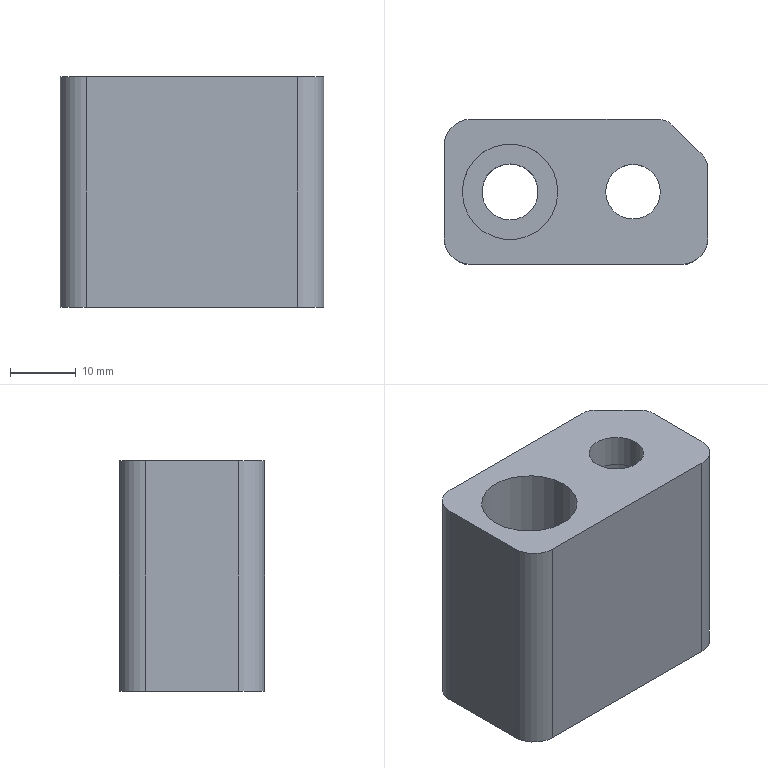Part | NX | features DIE-12 2 | 1 solid | 18 faces | box 40 x 22 x 35 mm | volume 23788 mm3 | plane 9 | cylinder 9 | commonest cylinder face diameters 8 x3 6 x2 8.29 x1 8.506 x1 10.29 x1 14.5 x1
STEP:
#1=CARTESIAN_POINT('',(2372.048,-869.122,858.716));
#2=VERTEX_POINT('',#1);
#3=CARTESIAN_POINT('',(2372.048,-869.122,823.716));
#4=VERTEX_POINT('',#3);
#5=CARTESIAN_POINT('',(2372.048,-869.122,858.716));
#6=DIRECTION('',(0.,0.,1.));
#7=VECTOR('',#6,1000.);
#8=LINE('',#5,#7);
#9=EDGE_CURVE('',#2,#4,#8,.F.);
#10=ORIENTED_EDGE('',*,*,#9,.T.);
#11=CARTESIAN_POINT('',(2404.048,-869.122,823.716));
#12=VERTEX_POINT('',#11);
#13=CARTESIAN_POINT('',(2387.048,-869.122,823.716));
#14=DIRECTION('',(1.,0.,0.));
#15=VECTOR('',#14,1000.);
#16=LINE('',#13,#15);
#17=EDGE_CURVE('',#4,#12,#16,.T.);
#18=ORIENTED_EDGE('',*,*,#17,.T.);
#19=CARTESIAN_POINT('',(2404.048,-869.122,858.716));
#20=VERTEX_POINT('',#19);
#21=CARTESIAN_POINT('',(2404.048,-869.122,858.716));
#22=DIRECTION('',(0.,0.,1.));
#23=VECTOR('',#22,1000.);
#24=LINE('',#21,#23);
#25=EDGE_CURVE('',#12,#20,#24,.T.);
#26=ORIENTED_EDGE('',*,*,#25,.T.);
#27=CARTESIAN_POINT('',(2387.048,-869.122,858.716));
#28=DIRECTION('',(-1.,0.,0.));
#29=VECTOR('',#28,1000.);
#30=LINE('',#27,#29);
#31=EDGE_CURVE('',#20,#2,#30,.T.);
#32=ORIENTED_EDGE('',*,*,#31,.T.);
#33=EDGE_LOOP('',(#10,#18,#26,#32));
#34=FACE_BOUND('',#33,.T.);
#35=CARTESIAN_POINT('',(2387.048,-869.122,858.716));
#36=DIRECTION('',(0.,-1.,0.));
#37=DIRECTION('',(0.,0.,1.));
#38=AXIS2_PLACEMENT_3D('',#35,#36,#37);
#39=PLANE('',#38);
#40=ADVANCED_FACE('',(#34),#39,.T.);
#41=CARTESIAN_POINT('',(2408.048,-865.122,858.716));
#42=VERTEX_POINT('',#41);
#43=CARTESIAN_POINT('',(2408.048,-865.122,823.716));
#44=VERTEX_POINT('',#43);
#45=CARTESIAN_POINT('',(2408.048,-865.122,858.716));
#46=DIRECTION('',(0.,0.,-1.));
#47=VECTOR('',#46,1000.);
#48=LINE('',#45,#47);
#49=EDGE_CURVE('',#42,#44,#48,.T.);
#50=ORIENTED_EDGE('',*,*,#49,.T.);
#51=CARTESIAN_POINT('',(2408.048,-854.658,823.716));
#52=VERTEX_POINT('',#51);
#53=CARTESIAN_POINT('',(2408.048,-858.122,823.716));
#54=DIRECTION('',(0.,1.,0.));
#55=VECTOR('',#54,1000.);
#56=LINE('',#53,#55);
#57=EDGE_CURVE('',#44,#52,#56,.T.);
#58=ORIENTED_EDGE('',*,*,#57,.T.);
#59=CARTESIAN_POINT('',(2408.048,-854.658,858.716));
#60=VERTEX_POINT('',#59);
#61=CARTESIAN_POINT('',(2408.048,-854.658,858.716));
#62=DIRECTION('',(0.,0.,-1.));
#63=VECTOR('',#62,1000.);
#64=LINE('',#61,#63);
#65=EDGE_CURVE('',#60,#52,#64,.T.);
#66=ORIENTED_EDGE('',*,*,#65,.F.);
#67=CARTESIAN_POINT('',(2408.048,-858.122,858.716));
#68=DIRECTION('',(0.,-1.,0.));
#69=VECTOR('',#68,1000.);
#70=LINE('',#67,#69);
#71=EDGE_CURVE('',#60,#42,#70,.T.);
#72=ORIENTED_EDGE('',*,*,#71,.T.);
#73=EDGE_LOOP('',(#50,#58,#66,#72));
#74=FACE_BOUND('',#73,.T.);
#75=CARTESIAN_POINT('',(2408.048,-858.122,858.716));
#76=DIRECTION('',(1.,0.,0.));
#77=DIRECTION('',(0.,0.,-1.));
#78=AXIS2_PLACEMENT_3D('',#75,#76,#77);
#79=PLANE('',#78);
#80=ADVANCED_FACE('',(#74),#79,.T.);
#81=CARTESIAN_POINT('',(2400.513,-847.122,823.716));
#82=VERTEX_POINT('',#81);
#83=CARTESIAN_POINT('',(2400.513,-847.122,858.716));
#84=VERTEX_POINT('',#83);
#85=CARTESIAN_POINT('',(2400.513,-847.122,858.716));
#86=DIRECTION('',(0.,0.,1.));
#87=VECTOR('',#86,1000.);
#88=LINE('',#85,#87);
#89=EDGE_CURVE('',#82,#84,#88,.T.);
#90=ORIENTED_EDGE('',*,*,#89,.F.);
#91=CARTESIAN_POINT('',(2372.048,-847.122,823.716));
#92=VERTEX_POINT('',#91);
#93=CARTESIAN_POINT('',(2387.048,-847.122,823.716));
#94=DIRECTION('',(-1.,0.,0.));
#95=VECTOR('',#94,1000.);
#96=LINE('',#93,#95);
#97=EDGE_CURVE('',#82,#92,#96,.T.);
#98=ORIENTED_EDGE('',*,*,#97,.T.);
#99=CARTESIAN_POINT('',(2372.048,-847.122,858.716));
#100=VERTEX_POINT('',#99);
#101=CARTESIAN_POINT('',(2372.048,-847.122,858.716));
#102=DIRECTION('',(0.,0.,-1.));
#103=VECTOR('',#102,1000.);
#104=LINE('',#101,#103);
#105=EDGE_CURVE('',#92,#100,#104,.F.);
#106=ORIENTED_EDGE('',*,*,#105,.T.);
#107=CARTESIAN_POINT('',(2387.048,-847.122,858.716));
#108=DIRECTION('',(1.,0.,0.));
#109=VECTOR('',#108,1000.);
#110=LINE('',#107,#109);
#111=EDGE_CURVE('',#100,#84,#110,.T.);
#112=ORIENTED_EDGE('',*,*,#111,.T.);
#113=EDGE_LOOP('',(#90,#98,#106,#112));
#114=FACE_BOUND('',#113,.T.);
#115=CARTESIAN_POINT('',(2387.048,-847.122,858.716));
#116=DIRECTION('',(0.,1.,0.));
#117=DIRECTION('',(0.,0.,-1.));
#118=AXIS2_PLACEMENT_3D('',#115,#116,#117);
#119=PLANE('',#118);
#120=ADVANCED_FACE('',(#114),#119,.T.);
#121=CARTESIAN_POINT('',(2368.048,-851.122,858.716));
#122=VERTEX_POINT('',#121);
#123=CARTESIAN_POINT('',(2368.048,-851.122,823.716));
#124=VERTEX_POINT('',#123);
#125=CARTESIAN_POINT('',(2368.048,-851.122,858.716));
#126=DIRECTION('',(0.,0.,1.));
#127=VECTOR('',#126,1000.);
#128=LINE('',#125,#127);
#129=EDGE_CURVE('',#122,#124,#128,.F.);
#130=ORIENTED_EDGE('',*,*,#129,.T.);
#131=CARTESIAN_POINT('',(2368.048,-865.122,823.716));
#132=VERTEX_POINT('',#131);
#133=CARTESIAN_POINT('',(2368.048,-858.122,823.716));
#134=DIRECTION('',(0.,-1.,0.));
#135=VECTOR('',#134,1000.);
#136=LINE('',#133,#135);
#137=EDGE_CURVE('',#124,#132,#136,.T.);
#138=ORIENTED_EDGE('',*,*,#137,.T.);
#139=CARTESIAN_POINT('',(2368.048,-865.122,858.716));
#140=VERTEX_POINT('',#139);
#141=CARTESIAN_POINT('',(2368.048,-865.122,858.716));
#142=DIRECTION('',(0.,0.,1.));
#143=VECTOR('',#142,1000.);
#144=LINE('',#141,#143);
#145=EDGE_CURVE('',#132,#140,#144,.T.);
#146=ORIENTED_EDGE('',*,*,#145,.T.);
#147=CARTESIAN_POINT('',(2368.048,-858.122,858.716));
#148=DIRECTION('',(0.,1.,0.));
#149=VECTOR('',#148,1000.);
#150=LINE('',#147,#149);
#151=EDGE_CURVE('',#140,#122,#150,.T.);
#152=ORIENTED_EDGE('',*,*,#151,.T.);
#153=EDGE_LOOP('',(#130,#138,#146,#152));
#154=FACE_BOUND('',#153,.T.);
#155=CARTESIAN_POINT('',(2368.048,-858.122,858.716));
#156=DIRECTION('',(-1.,0.,0.));
#157=DIRECTION('',(0.,0.,1.));
#158=AXIS2_PLACEMENT_3D('',#155,#156,#157);
#159=PLANE('',#158);
#160=ADVANCED_FACE('',(#154),#159,.T.);
#161=CARTESIAN_POINT('',(2407.17,-852.537,823.716));
#162=VERTEX_POINT('',#161);
#163=CARTESIAN_POINT('',(2407.17,-852.537,858.716));
#164=VERTEX_POINT('',#163);
#165=CARTESIAN_POINT('',(2407.17,-852.537,858.716));
#166=DIRECTION('',(0.,0.,-1.));
#167=VECTOR('',#166,1000.);
#168=LINE('',#165,#167);
#169=EDGE_CURVE('',#162,#164,#168,.F.);
#170=ORIENTED_EDGE('',*,*,#169,.F.);
#171=CARTESIAN_POINT('',(2402.634,-848.001,823.716));
#172=VERTEX_POINT('',#171);
#173=CARTESIAN_POINT('',(2399.902,-845.269,823.716));
#174=DIRECTION('',(-0.7071,0.7071,0.));
#175=VECTOR('',#174,1000.);
#176=LINE('',#173,#175);
#177=EDGE_CURVE('',#172,#162,#176,.F.);
#178=ORIENTED_EDGE('',*,*,#177,.F.);
#179=CARTESIAN_POINT('',(2402.634,-848.001,858.716));
#180=VERTEX_POINT('',#179);
#181=CARTESIAN_POINT('',(2402.634,-848.001,858.716));
#182=DIRECTION('',(0.,0.,1.));
#183=VECTOR('',#182,1000.);
#184=LINE('',#181,#183);
#185=EDGE_CURVE('',#180,#172,#184,.F.);
#186=ORIENTED_EDGE('',*,*,#185,.F.);
#187=CARTESIAN_POINT('',(2399.902,-845.269,858.716));
#188=DIRECTION('',(0.7071,-0.7071,0.));
#189=VECTOR('',#188,1000.);
#190=LINE('',#187,#189);
#191=EDGE_CURVE('',#164,#180,#190,.F.);
#192=ORIENTED_EDGE('',*,*,#191,.F.);
#193=EDGE_LOOP('',(#170,#178,#186,#192));
#194=FACE_BOUND('',#193,.T.);
#195=CARTESIAN_POINT('',(2402.402,-847.769,858.716));
#196=DIRECTION('',(-0.7071,-0.7071,0.));
#197=DIRECTION('',(-0.7071,0.7071,0.));
#198=AXIS2_PLACEMENT_3D('',#195,#196,#197);
#199=PLANE('',#198);
#200=ADVANCED_FACE('',(#194),#199,.F.);
#201=ORIENTED_EDGE('',*,*,#105,.F.);
#202=CARTESIAN_POINT('',(2372.048,-851.122,823.716));
#203=DIRECTION('',(0.,0.,-1.));
#204=DIRECTION('',(-1.,0.,0.));
#205=AXIS2_PLACEMENT_3D('',#202,#203,#204);
#206=CIRCLE('',#205,4.);
#207=EDGE_CURVE('',#124,#92,#206,.T.);
#208=ORIENTED_EDGE('',*,*,#207,.F.);
#209=ORIENTED_EDGE('',*,*,#129,.F.);
#210=CARTESIAN_POINT('',(2372.048,-851.122,858.716));
#211=DIRECTION('',(0.,0.,1.));
#212=DIRECTION('',(1.,0.,0.));
#213=AXIS2_PLACEMENT_3D('',#210,#211,#212);
#214=CIRCLE('',#213,4.);
#215=EDGE_CURVE('',#100,#122,#214,.T.);
#216=ORIENTED_EDGE('',*,*,#215,.F.);
#217=EDGE_LOOP('',(#201,#208,#209,#216));
#218=FACE_BOUND('',#217,.T.);
#219=CARTESIAN_POINT('',(2372.048,-851.122,858.716));
#220=DIRECTION('',(0.,0.,-1.));
#221=DIRECTION('',(0.,-1.,0.));
#222=AXIS2_PLACEMENT_3D('',#219,#220,#221);
#223=CYLINDRICAL_SURFACE('',#222,4.);
#224=ADVANCED_FACE('',(#218),#223,.T.);
#225=ORIENTED_EDGE('',*,*,#145,.F.);
#226=CARTESIAN_POINT('',(2372.048,-865.122,823.716));
#227=DIRECTION('',(0.,0.,-1.));
#228=DIRECTION('',(-1.,0.,0.));
#229=AXIS2_PLACEMENT_3D('',#226,#227,#228);
#230=CIRCLE('',#229,4.);
#231=EDGE_CURVE('',#4,#132,#230,.T.);
#232=ORIENTED_EDGE('',*,*,#231,.F.);
#233=ORIENTED_EDGE('',*,*,#9,.F.);
#234=CARTESIAN_POINT('',(2372.048,-865.122,858.716));
#235=DIRECTION('',(0.,0.,1.));
#236=DIRECTION('',(1.,0.,0.));
#237=AXIS2_PLACEMENT_3D('',#234,#235,#236);
#238=CIRCLE('',#237,4.);
#239=EDGE_CURVE('',#140,#2,#238,.T.);
#240=ORIENTED_EDGE('',*,*,#239,.F.);
#241=EDGE_LOOP('',(#225,#232,#233,#240));
#242=FACE_BOUND('',#241,.T.);
#243=CARTESIAN_POINT('',(2372.048,-865.122,858.716));
#244=DIRECTION('',(0.,0.,-1.));
#245=DIRECTION('',(0.,-1.,0.));
#246=AXIS2_PLACEMENT_3D('',#243,#244,#245);
#247=CYLINDRICAL_SURFACE('',#246,4.);
#248=ADVANCED_FACE('',(#242),#247,.T.);
#249=ORIENTED_EDGE('',*,*,#25,.F.);
#250=CARTESIAN_POINT('',(2404.048,-865.122,823.716));
#251=DIRECTION('',(0.,0.,-1.));
#252=DIRECTION('',(-1.,0.,0.));
#253=AXIS2_PLACEMENT_3D('',#250,#251,#252);
#254=CIRCLE('',#253,4.);
#255=EDGE_CURVE('',#44,#12,#254,.T.);
#256=ORIENTED_EDGE('',*,*,#255,.F.);
#257=ORIENTED_EDGE('',*,*,#49,.F.);
#258=CARTESIAN_POINT('',(2404.048,-865.122,858.716));
#259=DIRECTION('',(0.,0.,1.));
#260=DIRECTION('',(1.,0.,0.));
#261=AXIS2_PLACEMENT_3D('',#258,#259,#260);
#262=CIRCLE('',#261,4.);
#263=EDGE_CURVE('',#20,#42,#262,.T.);
#264=ORIENTED_EDGE('',*,*,#263,.F.);
#265=EDGE_LOOP('',(#249,#256,#257,#264));
#266=FACE_BOUND('',#265,.T.);
#267=CARTESIAN_POINT('',(2404.048,-865.122,858.716));
#268=DIRECTION('',(0.,0.,-1.));
#269=DIRECTION('',(0.,-1.,0.));
#270=AXIS2_PLACEMENT_3D('',#267,#268,#269);
#271=CYLINDRICAL_SURFACE('',#270,4.);
#272=ADVANCED_FACE('',(#266),#271,.T.);
#273=CARTESIAN_POINT('',(2385.298,-858.122,847.716));
#274=VERTEX_POINT('',#273);
#275=CARTESIAN_POINT('',(2378.048,-858.122,847.716));
#276=DIRECTION('',(0.,0.,1.));
#277=DIRECTION('',(1.,0.,0.));
#278=AXIS2_PLACEMENT_3D('',#275,#276,#277);
#279=CIRCLE('',#278,7.25);
#280=EDGE_CURVE('',#274,#274,#279,.F.);
#281=ORIENTED_EDGE('',*,*,#280,.T.);
#282=EDGE_LOOP('',(#281));
#283=FACE_BOUND('',#282,.T.);
#284=CARTESIAN_POINT('',(2385.298,-858.122,858.716));
#285=VERTEX_POINT('',#284);
#286=CARTESIAN_POINT('',(2378.048,-858.122,858.716));
#287=DIRECTION('',(0.,0.,-1.));
#288=DIRECTION('',(1.,0.,0.));
#289=AXIS2_PLACEMENT_3D('',#286,#287,#288);
#290=CIRCLE('',#289,7.25);
#291=EDGE_CURVE('',#285,#285,#290,.T.);
#292=ORIENTED_EDGE('',*,*,#291,.F.);
#293=EDGE_LOOP('',(#292));
#294=FACE_BOUND('',#293,.T.);
#295=CARTESIAN_POINT('',(2378.048,-858.122,847.716));
#296=DIRECTION('',(0.,0.,1.));
#297=DIRECTION('',(1.,0.,0.));
#298=AXIS2_PLACEMENT_3D('',#295,#296,#297);
#299=CYLINDRICAL_SURFACE('',#298,7.25);
#300=ADVANCED_FACE('',(#283,#294),#299,.F.);
#301=CARTESIAN_POINT('',(2391.553,-858.122,823.716));
#302=VERTEX_POINT('',#301);
#303=CARTESIAN_POINT('',(2396.698,-858.122,823.716));
#304=DIRECTION('',(0.,0.,-1.));
#305=DIRECTION('',(-1.,0.,0.));
#306=AXIS2_PLACEMENT_3D('',#303,#304,#305);
#307=CIRCLE('',#306,5.145);
#308=EDGE_CURVE('',#302,#302,#307,.T.);
#309=ORIENTED_EDGE('',*,*,#308,.T.);
#310=EDGE_LOOP('',(#309));
#311=FACE_BOUND('',#310,.T.);
#312=CARTESIAN_POINT('',(2401.843,-858.122,853.716));
#313=VERTEX_POINT('',#312);
#314=CARTESIAN_POINT('',(2396.698,-858.122,853.716));
#315=DIRECTION('',(0.,0.,1.));
#316=DIRECTION('',(1.,0.,0.));
#317=AXIS2_PLACEMENT_3D('',#314,#315,#316);
#318=CIRCLE('',#317,5.145);
#319=EDGE_CURVE('',#313,#313,#318,.F.);
#320=ORIENTED_EDGE('',*,*,#319,.F.);
#321=EDGE_LOOP('',(#320));
#322=FACE_BOUND('',#321,.T.);
#323=CARTESIAN_POINT('',(2396.698,-858.122,858.716));
#324=DIRECTION('',(0.,0.,-1.));
#325=DIRECTION('',(0.,-1.,0.));
#326=AXIS2_PLACEMENT_3D('',#323,#324,#325);
#327=CYLINDRICAL_SURFACE('',#326,5.145);
#328=ADVANCED_FACE('',(#311,#322),#327,.F.);
#329=ORIENTED_EDGE('',*,*,#185,.T.);
#330=CARTESIAN_POINT('',(2400.513,-850.122,823.716));
#331=DIRECTION('',(0.,0.,-1.));
#332=DIRECTION('',(-1.,0.,0.));
#333=AXIS2_PLACEMENT_3D('',#330,#331,#332);
#334=CIRCLE('',#333,3.);
#335=EDGE_CURVE('',#172,#82,#334,.F.);
#336=ORIENTED_EDGE('',*,*,#335,.T.);
#337=ORIENTED_EDGE('',*,*,#89,.T.);
#338=CARTESIAN_POINT('',(2400.513,-850.122,858.716));
#339=DIRECTION('',(0.,0.,1.));
#340=DIRECTION('',(1.,0.,0.));
#341=AXIS2_PLACEMENT_3D('',#338,#339,#340);
#342=CIRCLE('',#341,3.);
#343=EDGE_CURVE('',#84,#180,#342,.F.);
#344=ORIENTED_EDGE('',*,*,#343,.T.);
#345=EDGE_LOOP('',(#329,#336,#337,#344));
#346=FACE_BOUND('',#345,.T.);
#347=CARTESIAN_POINT('',(2400.513,-850.122,858.716));
#348=DIRECTION('',(0.,0.,1.));
#349=DIRECTION('',(0.,-1.,0.));
#350=AXIS2_PLACEMENT_3D('',#347,#348,#349);
#351=CYLINDRICAL_SURFACE('',#350,3.);
#352=ADVANCED_FACE('',(#346),#351,.T.);
#353=ORIENTED_EDGE('',*,*,#65,.T.);
#354=CARTESIAN_POINT('',(2405.048,-854.658,823.716));
#355=DIRECTION('',(0.,0.,-1.));
#356=DIRECTION('',(-1.,0.,0.));
#357=AXIS2_PLACEMENT_3D('',#354,#355,#356);
#358=CIRCLE('',#357,3.);
#359=EDGE_CURVE('',#52,#162,#358,.F.);
#360=ORIENTED_EDGE('',*,*,#359,.T.);
#361=ORIENTED_EDGE('',*,*,#169,.T.);
#362=CARTESIAN_POINT('',(2405.048,-854.658,858.716));
#363=DIRECTION('',(0.,0.,1.));
#364=DIRECTION('',(1.,0.,0.));
#365=AXIS2_PLACEMENT_3D('',#362,#363,#364);
#366=CIRCLE('',#365,3.);
#367=EDGE_CURVE('',#164,#60,#366,.F.);
#368=ORIENTED_EDGE('',*,*,#367,.T.);
#369=EDGE_LOOP('',(#353,#360,#361,#368));
#370=FACE_BOUND('',#369,.T.);
#371=CARTESIAN_POINT('',(2405.048,-854.658,858.716));
#372=DIRECTION('',(0.,0.,-1.));
#373=DIRECTION('',(0.,1.,0.));
#374=AXIS2_PLACEMENT_3D('',#371,#372,#373);
#375=CYLINDRICAL_SURFACE('',#374,3.);
#376=ADVANCED_FACE('',(#370),#375,.T.);
#377=ORIENTED_EDGE('',*,*,#308,.F.);
#378=EDGE_LOOP('',(#377));
#379=FACE_BOUND('',#378,.T.);
#380=CARTESIAN_POINT('',(2378.048,-862.375,823.716));
#381=VERTEX_POINT('',#380);
#382=CARTESIAN_POINT('',(2378.048,-858.122,823.716));
#383=DIRECTION('',(0.,0.,-1.));
#384=DIRECTION('',(0.,-1.,0.));
#385=AXIS2_PLACEMENT_3D('',#382,#383,#384);
#386=CIRCLE('',#385,4.253);
#387=EDGE_CURVE('',#381,#381,#386,.T.);
#388=ORIENTED_EDGE('',*,*,#387,.F.);
#389=EDGE_LOOP('',(#388));
#390=FACE_BOUND('',#389,.T.);
#391=ORIENTED_EDGE('',*,*,#177,.T.);
#392=ORIENTED_EDGE('',*,*,#359,.F.);
#393=ORIENTED_EDGE('',*,*,#57,.F.);
#394=ORIENTED_EDGE('',*,*,#255,.T.);
#395=ORIENTED_EDGE('',*,*,#17,.F.);
#396=ORIENTED_EDGE('',*,*,#231,.T.);
#397=ORIENTED_EDGE('',*,*,#137,.F.);
#398=ORIENTED_EDGE('',*,*,#207,.T.);
#399=ORIENTED_EDGE('',*,*,#97,.F.);
#400=ORIENTED_EDGE('',*,*,#335,.F.);
#401=EDGE_LOOP('',(#391,#392,#393,#394,#395,#396,#397,#398,#399,#400));
#402=FACE_BOUND('',#401,.T.);
#403=CARTESIAN_POINT('',(2387.048,-858.122,823.716));
#404=DIRECTION('',(0.,0.,-1.));
#405=DIRECTION('',(-1.,0.,0.));
#406=AXIS2_PLACEMENT_3D('',#403,#404,#405);
#407=PLANE('',#406);
#408=ADVANCED_FACE('',(#379,#390,#402),#407,.T.);
#409=CARTESIAN_POINT('',(2378.048,-862.375,847.716));
#410=VERTEX_POINT('',#409);
#411=CARTESIAN_POINT('',(2378.048,-858.122,847.716));
#412=DIRECTION('',(0.,0.,-1.));
#413=DIRECTION('',(0.,-1.,0.));
#414=AXIS2_PLACEMENT_3D('',#411,#412,#413);
#415=CIRCLE('',#414,4.253);
#416=EDGE_CURVE('',#410,#410,#415,.T.);
#417=ORIENTED_EDGE('',*,*,#416,.T.);
#418=EDGE_LOOP('',(#417));
#419=FACE_BOUND('',#418,.T.);
#420=ORIENTED_EDGE('',*,*,#280,.F.);
#421=EDGE_LOOP('',(#420));
#422=FACE_BOUND('',#421,.T.);
#423=CARTESIAN_POINT('',(2378.048,-858.122,847.716));
#424=DIRECTION('',(0.,0.,-1.));
#425=DIRECTION('',(0.,-1.,0.));
#426=AXIS2_PLACEMENT_3D('',#423,#424,#425);
#427=PLANE('',#426);
#428=ADVANCED_FACE('',(#419,#422),#427,.F.);
#429=ORIENTED_EDGE('',*,*,#387,.T.);
#430=EDGE_LOOP('',(#429));
#431=FACE_BOUND('',#430,.T.);
#432=ORIENTED_EDGE('',*,*,#416,.F.);
#433=EDGE_LOOP('',(#432));
#434=FACE_BOUND('',#433,.T.);
#435=CARTESIAN_POINT('',(2378.048,-858.122,822.716));
#436=DIRECTION('',(0.,0.,1.));
#437=DIRECTION('',(1.,0.,0.));
#438=AXIS2_PLACEMENT_3D('',#435,#436,#437);
#439=CYLINDRICAL_SURFACE('',#438,4.253);
#440=ADVANCED_FACE('',(#431,#434),#439,.F.);
#441=CARTESIAN_POINT('',(2400.843,-858.122,853.716));
#442=VERTEX_POINT('',#441);
#443=CARTESIAN_POINT('',(2396.698,-858.122,853.716));
#444=DIRECTION('',(0.,0.,1.));
#445=DIRECTION('',(1.,0.,0.));
#446=AXIS2_PLACEMENT_3D('',#443,#444,#445);
#447=CIRCLE('',#446,4.145);
#448=EDGE_CURVE('',#442,#442,#447,.T.);
#449=ORIENTED_EDGE('',*,*,#448,.F.);
#450=EDGE_LOOP('',(#449));
#451=FACE_BOUND('',#450,.T.);
#452=CARTESIAN_POINT('',(2400.843,-858.122,858.716));
#453=VERTEX_POINT('',#452);
#454=CARTESIAN_POINT('',(2396.698,-858.122,858.716));
#455=DIRECTION('',(0.,0.,1.));
#456=DIRECTION('',(1.,0.,0.));
#457=AXIS2_PLACEMENT_3D('',#454,#455,#456);
#458=CIRCLE('',#457,4.145);
#459=EDGE_CURVE('',#453,#453,#458,.T.);
#460=ORIENTED_EDGE('',*,*,#459,.T.);
#461=EDGE_LOOP('',(#460));
#462=FACE_BOUND('',#461,.T.);
#463=CARTESIAN_POINT('',(2396.698,-858.122,858.716));
#464=DIRECTION('',(0.,0.,-1.));
#465=DIRECTION('',(0.,-1.,0.));
#466=AXIS2_PLACEMENT_3D('',#463,#464,#465);
#467=CYLINDRICAL_SURFACE('',#466,4.145);
#468=ADVANCED_FACE('',(#451,#462),#467,.F.);
#469=ORIENTED_EDGE('',*,*,#459,.F.);
#470=EDGE_LOOP('',(#469));
#471=FACE_BOUND('',#470,.T.);
#472=ORIENTED_EDGE('',*,*,#291,.T.);
#473=EDGE_LOOP('',(#472));
#474=FACE_BOUND('',#473,.T.);
#475=ORIENTED_EDGE('',*,*,#111,.F.);
#476=ORIENTED_EDGE('',*,*,#215,.T.);
#477=ORIENTED_EDGE('',*,*,#151,.F.);
#478=ORIENTED_EDGE('',*,*,#239,.T.);
#479=ORIENTED_EDGE('',*,*,#31,.F.);
#480=ORIENTED_EDGE('',*,*,#263,.T.);
#481=ORIENTED_EDGE('',*,*,#71,.F.);
#482=ORIENTED_EDGE('',*,*,#367,.F.);
#483=ORIENTED_EDGE('',*,*,#191,.T.);
#484=ORIENTED_EDGE('',*,*,#343,.F.);
#485=EDGE_LOOP('',(#475,#476,#477,#478,#479,#480,#481,#482,#483,#484));
#486=FACE_BOUND('',#485,.T.);
#487=CARTESIAN_POINT('',(2387.048,-858.122,858.716));
#488=DIRECTION('',(0.,0.,1.));
#489=DIRECTION('',(1.,0.,0.));
#490=AXIS2_PLACEMENT_3D('',#487,#488,#489);
#491=PLANE('',#490);
#492=ADVANCED_FACE('',(#471,#474,#486),#491,.T.);
#493=ORIENTED_EDGE('',*,*,#319,.T.);
#494=EDGE_LOOP('',(#493));
#495=FACE_BOUND('',#494,.T.);
#496=ORIENTED_EDGE('',*,*,#448,.T.);
#497=EDGE_LOOP('',(#496));
#498=FACE_BOUND('',#497,.T.);
#499=CARTESIAN_POINT('',(2388.048,-858.122,853.716));
#500=DIRECTION('',(0.,0.,1.));
#501=DIRECTION('',(0.,-1.,0.));
#502=AXIS2_PLACEMENT_3D('',#499,#500,#501);
#503=PLANE('',#502);
#504=ADVANCED_FACE('',(#495,#498),#503,.F.);
#505=CLOSED_SHELL('',(#40,#80,#120,#160,#200,#224,#248,#272,#300,#328,#352,#376,#408,#428,#440,#468,#492,#504));
#506=MANIFOLD_SOLID_BREP('',#505);
#507=(LENGTH_UNIT()NAMED_UNIT(*)SI_UNIT(.MILLI.,.METRE.));
#508=UNCERTAINTY_MEASURE_WITH_UNIT(LENGTH_MEASURE(0.00001),#507,'','');
#509=(NAMED_UNIT(*)PLANE_ANGLE_UNIT()SI_UNIT($,.RADIAN.));
#510=(NAMED_UNIT(*)SI_UNIT($,.STERADIAN.)SOLID_ANGLE_UNIT());
#511=(GEOMETRIC_REPRESENTATION_CONTEXT(3)GLOBAL_UNCERTAINTY_ASSIGNED_CONTEXT((#508))GLOBAL_UNIT_ASSIGNED_CONTEXT((#507,#509,#510))REPRESENTATION_CONTEXT('',''));
#512=ADVANCED_BREP_SHAPE_REPRESENTATION('',(#506),#511);